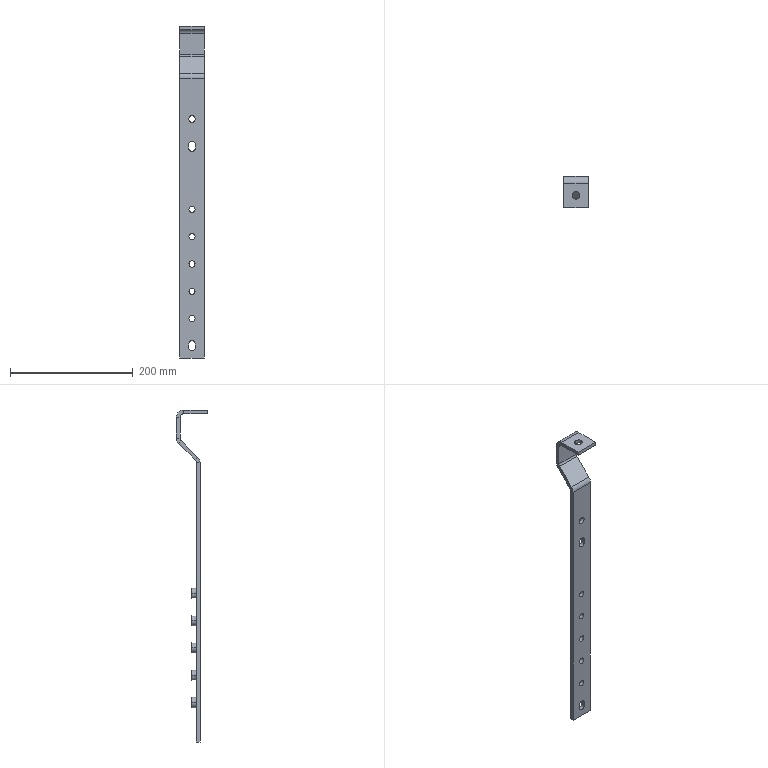Part | STEP file | 64806017 | 1 solid | 67 faces | box 40 x 51 x 542 mm | volume 142711 mm3 | cylinder 34 | plane 33 | commonest cylinder face diameters 10 x10 16.5 x10 11 x6 12 x3 24 x3 13 x2